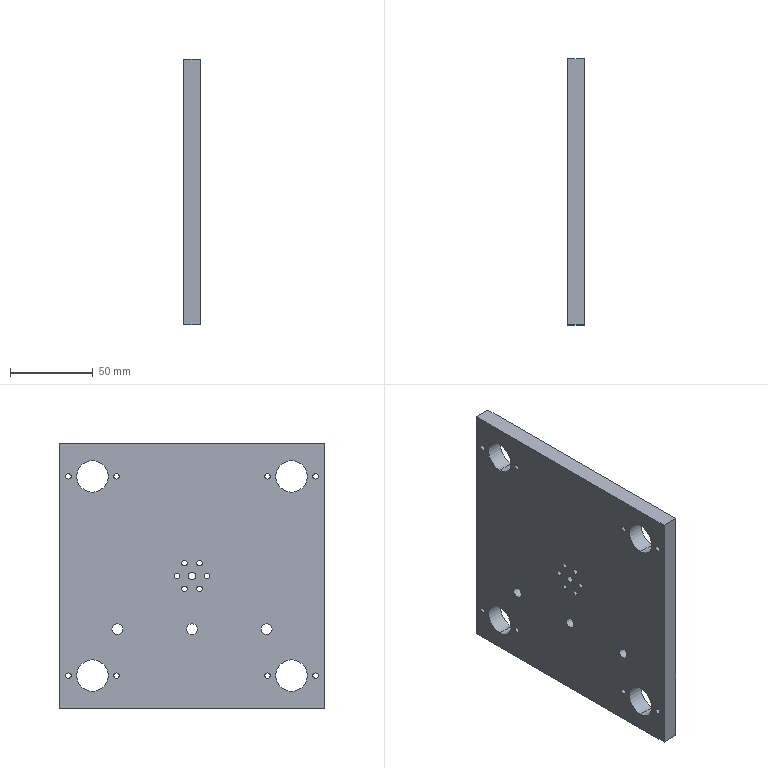Part | STEP file | 04-19 Up-down slide plate | 1 solid | 56 faces | box 10 x 160 x 160 mm | volume 241978 mm3 | cylinder 47 | plane 9 | commonest cylinder face diameters 3.3 x28 19 x8 6.5 x6 7.5 x3 4.5 x2